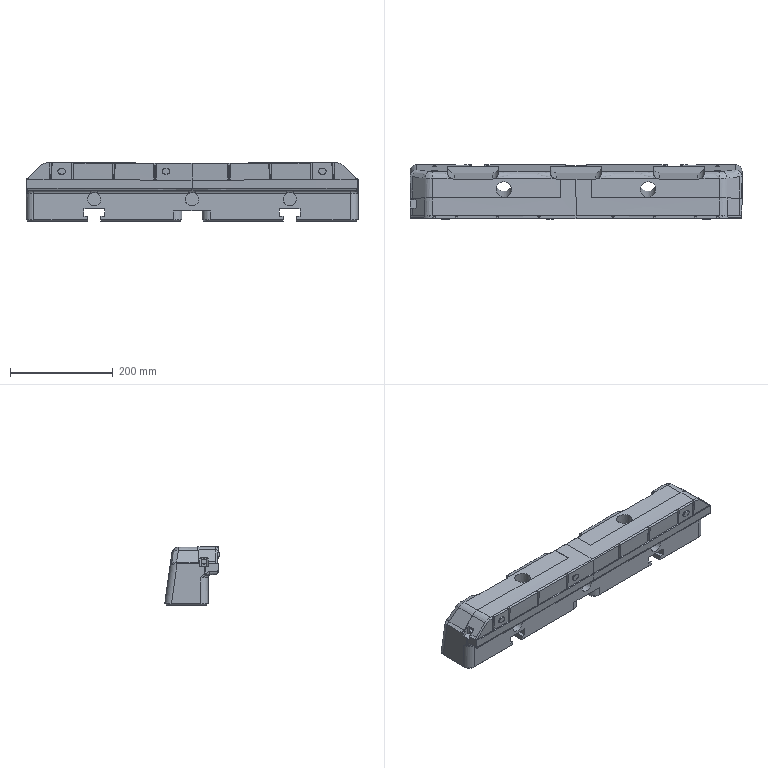Part | STEP file | solid 224 | 1 solid | 243 faces | box 645.466 x 105.916 x 113.789 mm | volume 5298019 mm3 | spline 106 | plane 74 | cylinder 50 | other 9 | cone 4 | commonest cylinder face diameters 10 x23 26 x11 6 x6 30 x6 12 x2 90 x2